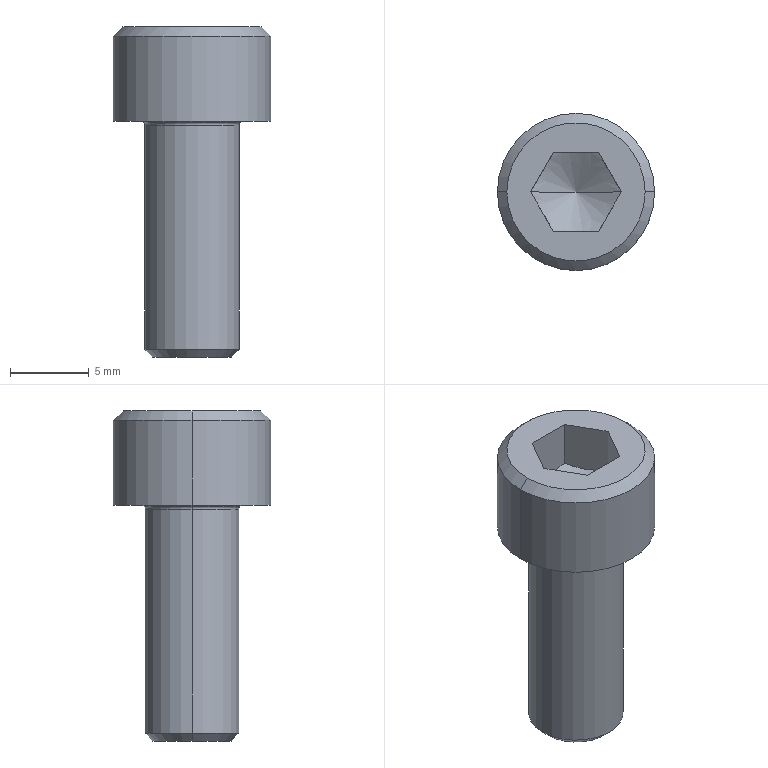Part | Creo | 1 solid | 23 faces | box 10 x 10 x 21 mm | volume 808.86 mm3 | plane 9 | cone 6 | cylinder 4 | torus 4 | commonest cylinder face diameters 6 x2 10 x2
STEP:
#1=CARTESIAN_POINT('',(0.,0.,0.));
#2=DIRECTION('',(0.,0.,1.));
#3=DIRECTION('',(1.,0.,0.));
#4=AXIS2_PLACEMENT_3D('',#1,#2,#3);
#5=CARTESIAN_POINT('',(-133.613,-0.4,-26.828));
#6=VERTEX_POINT('',#5);
#7=CARTESIAN_POINT('',(-135.057,2.1,-26.828));
#8=VERTEX_POINT('',#7);
#9=CARTESIAN_POINT('',(-133.613,-0.4,-26.828));
#10=CARTESIAN_POINT('',(-133.649,-0.3372,-26.848));
#11=CARTESIAN_POINT('',(-133.721,-0.2135,-26.887));
#12=CARTESIAN_POINT('',(-133.824,-0.03475,-26.936));
#13=CARTESIAN_POINT('',(-133.926,0.1409,-26.977));
#14=CARTESIAN_POINT('',(-134.026,0.3156,-27.009));
#15=CARTESIAN_POINT('',(-134.128,0.4922,-27.033));
#16=CARTESIAN_POINT('',(-134.231,0.6704,-27.047));
#17=CARTESIAN_POINT('',(-134.335,0.85,-27.052));
#18=CARTESIAN_POINT('',(-134.439,1.03,-27.047));
#19=CARTESIAN_POINT('',(-134.542,1.208,-27.033));
#20=CARTESIAN_POINT('',(-134.643,1.384,-27.009));
#21=CARTESIAN_POINT('',(-134.744,1.559,-26.977));
#22=CARTESIAN_POINT('',(-134.846,1.735,-26.936));
#23=CARTESIAN_POINT('',(-134.949,1.914,-26.887));
#24=CARTESIAN_POINT('',(-135.02,2.037,-26.848));
#25=CARTESIAN_POINT('',(-135.057,2.1,-26.828));
#26=B_SPLINE_CURVE_WITH_KNOTS('',3,(#9,#10,#11,#12,#13,#14,#15,#16,#17,#18,#19,#20,#21,#22,#23,#24,#25),.UNSPECIFIED.,.F.,.F.,(4,1,1,1,1,1,1,1,1,1,1,1,1,1,4),(0.,0.07143,0.1429,0.2143,0.2857,0.3571,0.4286,0.5,0.5714,0.6429,0.7143,0.7857,0.8571,0.9286,1.),.UNSPECIFIED.);
#27=EDGE_CURVE('',#6,#8,#26,.T.);
#28=ORIENTED_EDGE('',*,*,#27,.F.);
#29=CARTESIAN_POINT('',(-136.5,-0.4,-28.494));
#30=VERTEX_POINT('',#29);
#31=CARTESIAN_POINT('',(-136.5,-0.4,-28.494));
#32=DIRECTION('',(0.866,0.,0.5));
#33=VECTOR('',#32,3.333);
#34=LINE('',#31,#33);
#35=EDGE_CURVE('',#30,#6,#34,.T.);
#36=ORIENTED_EDGE('',*,*,#35,.F.);
#37=CARTESIAN_POINT('',(-139.387,-0.4,-26.828));
#38=VERTEX_POINT('',#37);
#39=CARTESIAN_POINT('',(-136.5,-0.4,-28.494));
#40=DIRECTION('',(-0.866,0.,0.5));
#41=VECTOR('',#40,3.333);
#42=LINE('',#39,#41);
#43=EDGE_CURVE('',#30,#38,#42,.T.);
#44=ORIENTED_EDGE('',*,*,#43,.T.);
#45=CARTESIAN_POINT('',(-137.943,2.1,-26.828));
#46=VERTEX_POINT('',#45);
#47=CARTESIAN_POINT('',(-137.943,2.1,-26.828));
#48=CARTESIAN_POINT('',(-137.98,2.037,-26.848));
#49=CARTESIAN_POINT('',(-138.051,1.914,-26.887));
#50=CARTESIAN_POINT('',(-138.154,1.735,-26.936));
#51=CARTESIAN_POINT('',(-138.256,1.559,-26.977));
#52=CARTESIAN_POINT('',(-138.357,1.384,-27.009));
#53=CARTESIAN_POINT('',(-138.458,1.208,-27.033));
#54=CARTESIAN_POINT('',(-138.561,1.03,-27.047));
#55=CARTESIAN_POINT('',(-138.665,0.85,-27.052));
#56=CARTESIAN_POINT('',(-138.769,0.6704,-27.047));
#57=CARTESIAN_POINT('',(-138.872,0.4922,-27.033));
#58=CARTESIAN_POINT('',(-138.974,0.3156,-27.009));
#59=CARTESIAN_POINT('',(-139.074,0.1409,-26.977));
#60=CARTESIAN_POINT('',(-139.176,-0.03475,-26.936));
#61=CARTESIAN_POINT('',(-139.279,-0.2135,-26.887));
#62=CARTESIAN_POINT('',(-139.351,-0.3372,-26.848));
#63=CARTESIAN_POINT('',(-139.387,-0.4,-26.828));
#64=B_SPLINE_CURVE_WITH_KNOTS('',3,(#47,#48,#49,#50,#51,#52,#53,#54,#55,#56,#57,#58,#59,#60,#61,#62,#63),.UNSPECIFIED.,.F.,.F.,(4,1,1,1,1,1,1,1,1,1,1,1,1,1,4),(0.,0.07143,0.1429,0.2143,0.2857,0.3571,0.4286,0.5,0.5714,0.6429,0.7143,0.7857,0.8571,0.9286,1.),.UNSPECIFIED.);
#65=EDGE_CURVE('',#46,#38,#64,.T.);
#66=ORIENTED_EDGE('',*,*,#65,.F.);
#67=CARTESIAN_POINT('',(-135.057,2.1,-26.828));
#68=CARTESIAN_POINT('',(-135.129,2.1,-26.848));
#69=CARTESIAN_POINT('',(-135.272,2.1,-26.887));
#70=CARTESIAN_POINT('',(-135.478,2.1,-26.936));
#71=CARTESIAN_POINT('',(-135.68,2.1,-26.977));
#72=CARTESIAN_POINT('',(-135.882,2.1,-27.009));
#73=CARTESIAN_POINT('',(-136.086,2.1,-27.033));
#74=CARTESIAN_POINT('',(-136.292,2.1,-27.047));
#75=CARTESIAN_POINT('',(-136.5,2.1,-27.052));
#76=CARTESIAN_POINT('',(-136.708,2.1,-27.047));
#77=CARTESIAN_POINT('',(-136.914,2.1,-27.033));
#78=CARTESIAN_POINT('',(-137.118,2.1,-27.009));
#79=CARTESIAN_POINT('',(-137.32,2.1,-26.977));
#80=CARTESIAN_POINT('',(-137.522,2.1,-26.936));
#81=CARTESIAN_POINT('',(-137.728,2.1,-26.887));
#82=CARTESIAN_POINT('',(-137.871,2.1,-26.848));
#83=CARTESIAN_POINT('',(-137.943,2.1,-26.828));
#84=B_SPLINE_CURVE_WITH_KNOTS('',3,(#67,#68,#69,#70,#71,#72,#73,#74,#75,#76,#77,#78,#79,#80,#81,#82,#83),.UNSPECIFIED.,.F.,.F.,(4,1,1,1,1,1,1,1,1,1,1,1,1,1,4),(0.,0.07143,0.1429,0.2143,0.2857,0.3571,0.4286,0.5,0.5714,0.6429,0.7143,0.7857,0.8571,0.9286,1.),.UNSPECIFIED.);
#85=EDGE_CURVE('',#8,#46,#84,.T.);
#86=ORIENTED_EDGE('',*,*,#85,.F.);
#87=EDGE_LOOP('',(#28,#36,#44,#66,#86));
#88=FACE_OUTER_BOUND('',#87,.F.);
#89=CARTESIAN_POINT('',(-136.5,-0.4,-27.644));
#90=DIRECTION('',(0.,0.,1.));
#91=DIRECTION('',(1.,0.,0.));
#92=AXIS2_PLACEMENT_3D('',#89,#90,#91);
#93=CONICAL_SURFACE('',#92,1.472,60.);
#94=ADVANCED_FACE('',(#88),#93,.F.);
#95=CARTESIAN_POINT('',(-135.057,2.1,-23.828));
#96=VERTEX_POINT('',#95);
#97=CARTESIAN_POINT('',(-133.613,-0.4,-23.828));
#98=VERTEX_POINT('',#97);
#99=CARTESIAN_POINT('',(-135.057,2.1,-23.828));
#100=DIRECTION('',(0.5,-0.866,0.));
#101=VECTOR('',#100,2.887);
#102=LINE('',#99,#101);
#103=EDGE_CURVE('',#96,#98,#102,.T.);
#104=ORIENTED_EDGE('',*,*,#103,.T.);
#105=CARTESIAN_POINT('',(-133.613,-0.4,-23.828));
#106=DIRECTION('',(0.,0.,-1.));
#107=VECTOR('',#106,3.);
#108=LINE('',#105,#107);
#109=EDGE_CURVE('',#98,#6,#108,.T.);
#110=ORIENTED_EDGE('',*,*,#109,.T.);
#111=ORIENTED_EDGE('',*,*,#27,.T.);
#112=CARTESIAN_POINT('',(-135.057,2.1,-23.828));
#113=DIRECTION('',(0.,0.,-1.));
#114=VECTOR('',#113,3.);
#115=LINE('',#112,#114);
#116=EDGE_CURVE('',#96,#8,#115,.T.);
#117=ORIENTED_EDGE('',*,*,#116,.F.);
#118=EDGE_LOOP('',(#104,#110,#111,#117));
#119=FACE_OUTER_BOUND('',#118,.F.);
#120=CARTESIAN_POINT('',(-135.057,2.1,-26.828));
#121=DIRECTION('',(-0.866,-0.5,0.));
#122=DIRECTION('',(0.5,-0.866,0.));
#123=AXIS2_PLACEMENT_3D('',#120,#121,#122);
#124=PLANE('',#123);
#125=ADVANCED_FACE('',(#119),#124,.T.);
#126=CARTESIAN_POINT('',(-132.1,-0.4,-23.828));
#127=VERTEX_POINT('',#126);
#128=CARTESIAN_POINT('',(-140.9,-0.4,-23.828));
#129=VERTEX_POINT('',#128);
#130=CARTESIAN_POINT('',(-136.5,-0.4,-23.828));
#131=DIRECTION('',(0.,0.,1.));
#132=DIRECTION('',(1.,0.,0.));
#133=AXIS2_PLACEMENT_3D('',#130,#131,#132);
#134=CIRCLE('',#133,4.4);
#135=EDGE_CURVE('',#127,#129,#134,.T.);
#136=ORIENTED_EDGE('',*,*,#135,.F.);
#137=CARTESIAN_POINT('',(-136.5,-0.4,-23.828));
#138=DIRECTION('',(0.,0.,1.));
#139=DIRECTION('',(-1.,0.,0.));
#140=AXIS2_PLACEMENT_3D('',#137,#138,#139);
#141=CIRCLE('',#140,4.4);
#142=EDGE_CURVE('',#129,#127,#141,.T.);
#143=ORIENTED_EDGE('',*,*,#142,.F.);
#144=EDGE_LOOP('',(#136,#143));
#145=FACE_OUTER_BOUND('',#144,.F.);
#146=CARTESIAN_POINT('',(-135.057,-2.9,-23.828));
#147=VERTEX_POINT('',#146);
#148=CARTESIAN_POINT('',(-133.613,-0.4,-23.828));
#149=DIRECTION('',(-0.5,-0.866,0.));
#150=VECTOR('',#149,2.887);
#151=LINE('',#148,#150);
#152=EDGE_CURVE('',#98,#147,#151,.T.);
#153=ORIENTED_EDGE('',*,*,#152,.F.);
#154=ORIENTED_EDGE('',*,*,#103,.F.);
#155=CARTESIAN_POINT('',(-137.943,2.1,-23.828));
#156=VERTEX_POINT('',#155);
#157=CARTESIAN_POINT('',(-135.057,2.1,-23.828));
#158=DIRECTION('',(-1.,0.,0.));
#159=VECTOR('',#158,2.887);
#160=LINE('',#157,#159);
#161=EDGE_CURVE('',#96,#156,#160,.T.);
#162=ORIENTED_EDGE('',*,*,#161,.T.);
#163=CARTESIAN_POINT('',(-139.387,-0.4,-23.828));
#164=VERTEX_POINT('',#163);
#165=CARTESIAN_POINT('',(-139.387,-0.4,-23.828));
#166=DIRECTION('',(0.5,0.866,0.));
#167=VECTOR('',#166,2.887);
#168=LINE('',#165,#167);
#169=EDGE_CURVE('',#164,#156,#168,.T.);
#170=ORIENTED_EDGE('',*,*,#169,.F.);
#171=CARTESIAN_POINT('',(-137.943,-2.9,-23.828));
#172=VERTEX_POINT('',#171);
#173=CARTESIAN_POINT('',(-137.943,-2.9,-23.828));
#174=DIRECTION('',(-0.5,0.866,0.));
#175=VECTOR('',#174,2.887);
#176=LINE('',#173,#175);
#177=EDGE_CURVE('',#172,#164,#176,.T.);
#178=ORIENTED_EDGE('',*,*,#177,.F.);
#179=CARTESIAN_POINT('',(-137.943,-2.9,-23.828));
#180=DIRECTION('',(1.,0.,0.));
#181=VECTOR('',#180,2.887);
#182=LINE('',#179,#181);
#183=EDGE_CURVE('',#172,#147,#182,.T.);
#184=ORIENTED_EDGE('',*,*,#183,.T.);
#185=EDGE_LOOP('',(#153,#154,#162,#170,#178,#184));
#186=FACE_BOUND('',#185,.F.);
#187=CARTESIAN_POINT('',(-136.5,-0.4,-23.828));
#188=DIRECTION('',(0.,0.,1.));
#189=DIRECTION('',(1.,0.,0.));
#190=AXIS2_PLACEMENT_3D('',#187,#188,#189);
#191=PLANE('',#190);
#192=ADVANCED_FACE('',(#145,#186),#191,.T.);
#193=CARTESIAN_POINT('',(-131.5,-0.4,-24.427));
#194=VERTEX_POINT('',#193);
#195=CARTESIAN_POINT('',(-141.5,-0.4,-24.427));
#196=VERTEX_POINT('',#195);
#197=CARTESIAN_POINT('',(-136.5,-0.4,-24.427));
#198=DIRECTION('',(0.,0.,1.));
#199=DIRECTION('',(1.,0.,0.));
#200=AXIS2_PLACEMENT_3D('',#197,#198,#199);
#201=CIRCLE('',#200,5.);
#202=EDGE_CURVE('',#194,#196,#201,.T.);
#203=ORIENTED_EDGE('',*,*,#202,.F.);
#204=CARTESIAN_POINT('',(-132.1,-0.4,-23.828));
#205=DIRECTION('',(0.7071,0.,-0.7071));
#206=VECTOR('',#205,0.8485);
#207=LINE('',#204,#206);
#208=EDGE_CURVE('',#127,#194,#207,.T.);
#209=ORIENTED_EDGE('',*,*,#208,.F.);
#210=ORIENTED_EDGE('',*,*,#135,.T.);
#211=CARTESIAN_POINT('',(-140.9,-0.4,-23.828));
#212=DIRECTION('',(-0.7071,0.,-0.7071));
#213=VECTOR('',#212,0.8485);
#214=LINE('',#211,#213);
#215=EDGE_CURVE('',#129,#196,#214,.T.);
#216=ORIENTED_EDGE('',*,*,#215,.T.);
#217=EDGE_LOOP('',(#203,#209,#210,#216));
#218=FACE_OUTER_BOUND('',#217,.F.);
#219=CARTESIAN_POINT('',(-136.5,-0.4,-24.128));
#220=DIRECTION('',(0.,0.,-1.));
#221=DIRECTION('',(-1.,0.,0.));
#222=AXIS2_PLACEMENT_3D('',#219,#220,#221);
#223=CONICAL_SURFACE('',#222,4.7,45.);
#224=ADVANCED_FACE('',(#218),#223,.T.);
#225=ORIENTED_EDGE('',*,*,#202,.T.);
#226=CARTESIAN_POINT('',(-141.5,-0.4,-29.828));
#227=VERTEX_POINT('',#226);
#228=CARTESIAN_POINT('',(-141.5,-0.4,-29.828));
#229=DIRECTION('',(0.,0.,1.));
#230=VECTOR('',#229,5.4);
#231=LINE('',#228,#230);
#232=EDGE_CURVE('',#227,#196,#231,.T.);
#233=ORIENTED_EDGE('',*,*,#232,.F.);
#234=CARTESIAN_POINT('',(-131.5,-0.4,-29.828));
#235=VERTEX_POINT('',#234);
#236=CARTESIAN_POINT('',(-136.5,-0.4,-29.828));
#237=DIRECTION('',(0.,0.,-1.));
#238=DIRECTION('',(-1.,0.,0.));
#239=AXIS2_PLACEMENT_3D('',#236,#237,#238);
#240=CIRCLE('',#239,5.);
#241=EDGE_CURVE('',#227,#235,#240,.T.);
#242=ORIENTED_EDGE('',*,*,#241,.T.);
#243=CARTESIAN_POINT('',(-131.5,-0.4,-29.828));
#244=DIRECTION('',(0.,0.,1.));
#245=VECTOR('',#244,5.4);
#246=LINE('',#243,#245);
#247=EDGE_CURVE('',#235,#194,#246,.T.);
#248=ORIENTED_EDGE('',*,*,#247,.T.);
#249=EDGE_LOOP('',(#225,#233,#242,#248));
#250=FACE_OUTER_BOUND('',#249,.F.);
#251=CARTESIAN_POINT('',(-136.5,-0.4,-29.828));
#252=DIRECTION('',(0.,0.,1.));
#253=DIRECTION('',(1.,0.,0.));
#254=AXIS2_PLACEMENT_3D('',#251,#252,#253);
#255=CYLINDRICAL_SURFACE('',#254,5.);
#256=ADVANCED_FACE('',(#250),#255,.T.);
#257=CARTESIAN_POINT('',(-136.5,-0.4,-24.427));
#258=DIRECTION('',(0.,0.,1.));
#259=DIRECTION('',(-1.,0.,0.));
#260=AXIS2_PLACEMENT_3D('',#257,#258,#259);
#261=CIRCLE('',#260,5.);
#262=EDGE_CURVE('',#196,#194,#261,.T.);
#263=ORIENTED_EDGE('',*,*,#262,.T.);
#264=ORIENTED_EDGE('',*,*,#247,.F.);
#265=CARTESIAN_POINT('',(-136.5,-0.4,-29.828));
#266=DIRECTION('',(0.,0.,-1.));
#267=DIRECTION('',(1.,0.,0.));
#268=AXIS2_PLACEMENT_3D('',#265,#266,#267);
#269=CIRCLE('',#268,5.);
#270=EDGE_CURVE('',#235,#227,#269,.T.);
#271=ORIENTED_EDGE('',*,*,#270,.T.);
#272=ORIENTED_EDGE('',*,*,#232,.T.);
#273=EDGE_LOOP('',(#263,#264,#271,#272));
#274=FACE_OUTER_BOUND('',#273,.F.);
#275=CARTESIAN_POINT('',(-136.5,-0.4,-29.828));
#276=DIRECTION('',(0.,0.,1.));
#277=DIRECTION('',(1.,0.,0.));
#278=AXIS2_PLACEMENT_3D('',#275,#276,#277);
#279=CYLINDRICAL_SURFACE('',#278,5.);
#280=ADVANCED_FACE('',(#274),#279,.T.);
#281=ORIENTED_EDGE('',*,*,#262,.F.);
#282=ORIENTED_EDGE('',*,*,#215,.F.);
#283=ORIENTED_EDGE('',*,*,#142,.T.);
#284=ORIENTED_EDGE('',*,*,#208,.T.);
#285=EDGE_LOOP('',(#281,#282,#283,#284));
#286=FACE_OUTER_BOUND('',#285,.F.);
#287=CARTESIAN_POINT('',(-136.5,-0.4,-24.128));
#288=DIRECTION('',(0.,0.,-1.));
#289=DIRECTION('',(-1.,0.,0.));
#290=AXIS2_PLACEMENT_3D('',#287,#288,#289);
#291=CONICAL_SURFACE('',#290,4.7,45.);
#292=ADVANCED_FACE('',(#286),#291,.T.);
#293=ORIENTED_EDGE('',*,*,#270,.F.);
#294=ORIENTED_EDGE('',*,*,#241,.F.);
#295=EDGE_LOOP('',(#293,#294));
#296=FACE_OUTER_BOUND('',#295,.F.);
#297=CARTESIAN_POINT('',(-133.25,-0.4,-29.828));
#298=VERTEX_POINT('',#297);
#299=CARTESIAN_POINT('',(-139.75,-0.4,-29.828));
#300=VERTEX_POINT('',#299);
#301=CARTESIAN_POINT('',(-136.5,-0.4,-29.828));
#302=DIRECTION('',(0.,0.,1.));
#303=DIRECTION('',(1.,0.,0.));
#304=AXIS2_PLACEMENT_3D('',#301,#302,#303);
#305=CIRCLE('',#304,3.25);
#306=EDGE_CURVE('',#298,#300,#305,.T.);
#307=ORIENTED_EDGE('',*,*,#306,.F.);
#308=CARTESIAN_POINT('',(-136.5,-0.4,-29.828));
#309=DIRECTION('',(0.,0.,1.));
#310=DIRECTION('',(-1.,0.,0.));
#311=AXIS2_PLACEMENT_3D('',#308,#309,#310);
#312=CIRCLE('',#311,3.25);
#313=EDGE_CURVE('',#300,#298,#312,.T.);
#314=ORIENTED_EDGE('',*,*,#313,.F.);
#315=EDGE_LOOP('',(#307,#314));
#316=FACE_BOUND('',#315,.F.);
#317=CARTESIAN_POINT('',(-136.5,-0.4,-29.828));
#318=DIRECTION('',(0.,0.,1.));
#319=DIRECTION('',(1.,0.,0.));
#320=AXIS2_PLACEMENT_3D('',#317,#318,#319);
#321=PLANE('',#320);
#322=ADVANCED_FACE('',(#296,#316),#321,.F.);
#323=ORIENTED_EDGE('',*,*,#306,.T.);
#324=CARTESIAN_POINT('',(-139.573,-0.4,-29.901));
#325=VERTEX_POINT('',#324);
#326=CARTESIAN_POINT('',(-139.75,-0.4,-30.078));
#327=DIRECTION('',(0.,1.,0.));
#328=DIRECTION('',(0.,0.,1.));
#329=AXIS2_PLACEMENT_3D('',#326,#327,#328);
#330=CIRCLE('',#329,0.25);
#331=EDGE_CURVE('',#300,#325,#330,.T.);
#332=ORIENTED_EDGE('',*,*,#331,.T.);
#333=CARTESIAN_POINT('',(-133.427,-0.4,-29.901));
#334=VERTEX_POINT('',#333);
#335=CARTESIAN_POINT('',(-136.5,-0.4,-29.901));
#336=DIRECTION('',(0.,0.,1.));
#337=DIRECTION('',(1.,0.,0.));
#338=AXIS2_PLACEMENT_3D('',#335,#336,#337);
#339=CIRCLE('',#338,3.073);
#340=EDGE_CURVE('',#334,#325,#339,.T.);
#341=ORIENTED_EDGE('',*,*,#340,.F.);
#342=CARTESIAN_POINT('',(-133.25,-0.4,-30.078));
#343=DIRECTION('',(0.,-1.,0.));
#344=DIRECTION('',(0.,0.,1.));
#345=AXIS2_PLACEMENT_3D('',#342,#343,#344);
#346=CIRCLE('',#345,0.25);
#347=EDGE_CURVE('',#298,#334,#346,.T.);
#348=ORIENTED_EDGE('',*,*,#347,.F.);
#349=EDGE_LOOP('',(#323,#332,#341,#348));
#350=FACE_OUTER_BOUND('',#349,.F.);
#351=CARTESIAN_POINT('',(-136.5,-0.4,-30.078));
#352=DIRECTION('',(0.,0.,1.));
#353=DIRECTION('',(1.,0.,0.));
#354=AXIS2_PLACEMENT_3D('',#351,#352,#353);
#355=TOROIDAL_SURFACE('',#354,3.25,0.25);
#356=ADVANCED_FACE('',(#350),#355,.F.);
#357=ORIENTED_EDGE('',*,*,#313,.T.);
#358=ORIENTED_EDGE('',*,*,#347,.T.);
#359=CARTESIAN_POINT('',(-136.5,-0.4,-29.901));
#360=DIRECTION('',(0.,0.,1.));
#361=DIRECTION('',(-1.,0.,0.));
#362=AXIS2_PLACEMENT_3D('',#359,#360,#361);
#363=CIRCLE('',#362,3.073);
#364=EDGE_CURVE('',#325,#334,#363,.T.);
#365=ORIENTED_EDGE('',*,*,#364,.F.);
#366=ORIENTED_EDGE('',*,*,#331,.F.);
#367=EDGE_LOOP('',(#357,#358,#365,#366));
#368=FACE_OUTER_BOUND('',#367,.F.);
#369=CARTESIAN_POINT('',(-136.5,-0.4,-30.078));
#370=DIRECTION('',(0.,0.,1.));
#371=DIRECTION('',(1.,0.,0.));
#372=AXIS2_PLACEMENT_3D('',#369,#370,#371);
#373=TOROIDAL_SURFACE('',#372,3.25,0.25);
#374=ADVANCED_FACE('',(#368),#373,.F.);
#375=CARTESIAN_POINT('',(-139.5,-0.4,-30.078));
#376=VERTEX_POINT('',#375);
#377=CARTESIAN_POINT('',(-133.5,-0.4,-30.078));
#378=VERTEX_POINT('',#377);
#379=CARTESIAN_POINT('',(-136.5,-0.4,-30.078));
#380=DIRECTION('',(0.,0.,1.));
#381=DIRECTION('',(-1.,0.,0.));
#382=AXIS2_PLACEMENT_3D('',#379,#380,#381);
#383=CIRCLE('',#382,3.);
#384=EDGE_CURVE('',#376,#378,#383,.T.);
#385=ORIENTED_EDGE('',*,*,#384,.F.);
#386=CARTESIAN_POINT('',(-139.75,-0.4,-30.078));
#387=DIRECTION('',(0.,1.,0.));
#388=DIRECTION('',(0.7071,0.,0.7071));
#389=AXIS2_PLACEMENT_3D('',#386,#387,#388);
#390=CIRCLE('',#389,0.25);
#391=EDGE_CURVE('',#325,#376,#390,.T.);
#392=ORIENTED_EDGE('',*,*,#391,.F.);
#393=ORIENTED_EDGE('',*,*,#364,.T.);
#394=CARTESIAN_POINT('',(-133.25,-0.4,-30.078));
#395=DIRECTION('',(0.,-1.,0.));
#396=DIRECTION('',(-0.7071,0.,0.7071));
#397=AXIS2_PLACEMENT_3D('',#394,#395,#396);
#398=CIRCLE('',#397,0.25);
#399=EDGE_CURVE('',#334,#378,#398,.T.);
#400=ORIENTED_EDGE('',*,*,#399,.T.);
#401=EDGE_LOOP('',(#385,#392,#393,#400));
#402=FACE_OUTER_BOUND('',#401,.F.);
#403=CARTESIAN_POINT('',(-136.5,-0.4,-30.078));
#404=DIRECTION('',(0.,0.,1.));
#405=DIRECTION('',(1.,0.,0.));
#406=AXIS2_PLACEMENT_3D('',#403,#404,#405);
#407=TOROIDAL_SURFACE('',#406,3.25,0.25);
#408=ADVANCED_FACE('',(#402),#407,.F.);
#409=CARTESIAN_POINT('',(-133.5,-0.4,-44.328));
#410=VERTEX_POINT('',#409);
#411=CARTESIAN_POINT('',(-139.5,-0.4,-44.328));
#412=VERTEX_POINT('',#411);
#413=CARTESIAN_POINT('',(-136.5,-0.4,-44.328));
#414=DIRECTION('',(0.,0.,-1.));
#415=DIRECTION('',(1.,0.,0.));
#416=AXIS2_PLACEMENT_3D('',#413,#414,#415);
#417=CIRCLE('',#416,3.);
#418=EDGE_CURVE('',#410,#412,#417,.T.);
#419=ORIENTED_EDGE('',*,*,#418,.T.);
#420=CARTESIAN_POINT('',(-139.5,-0.4,-44.328));
#421=DIRECTION('',(0.,0.,1.));
#422=VECTOR('',#421,14.25);
#423=LINE('',#420,#422);
#424=EDGE_CURVE('',#412,#376,#423,.T.);
#425=ORIENTED_EDGE('',*,*,#424,.T.);
#426=ORIENTED_EDGE('',*,*,#384,.T.);
#427=CARTESIAN_POINT('',(-133.5,-0.4,-44.328));
#428=DIRECTION('',(0.,0.,1.));
#429=VECTOR('',#428,14.25);
#430=LINE('',#427,#429);
#431=EDGE_CURVE('',#410,#378,#430,.T.);
#432=ORIENTED_EDGE('',*,*,#431,.F.);
#433=EDGE_LOOP('',(#419,#425,#426,#432));
#434=FACE_OUTER_BOUND('',#433,.F.);
#435=CARTESIAN_POINT('',(-136.5,-0.4,-44.828));
#436=DIRECTION('',(0.,0.,1.));
#437=DIRECTION('',(1.,0.,0.));
#438=AXIS2_PLACEMENT_3D('',#435,#436,#437);
#439=CYLINDRICAL_SURFACE('',#438,3.);
#440=ADVANCED_FACE('',(#434),#439,.T.);
#441=CARTESIAN_POINT('',(-134.,-0.4,-44.828));
#442=VERTEX_POINT('',#441);
#443=CARTESIAN_POINT('',(-139.,-0.4,-44.828));
#444=VERTEX_POINT('',#443);
#445=CARTESIAN_POINT('',(-136.5,-0.4,-44.828));
#446=DIRECTION('',(0.,0.,-1.));
#447=DIRECTION('',(1.,0.,0.));
#448=AXIS2_PLACEMENT_3D('',#445,#446,#447);
#449=CIRCLE('',#448,2.5);
#450=EDGE_CURVE('',#442,#444,#449,.T.);
#451=ORIENTED_EDGE('',*,*,#450,.T.);
#452=CARTESIAN_POINT('',(-139.,-0.4,-44.828));
#453=DIRECTION('',(-0.7071,0.,0.7071));
#454=VECTOR('',#453,0.7071);
#455=LINE('',#452,#454);
#456=EDGE_CURVE('',#444,#412,#455,.T.);
#457=ORIENTED_EDGE('',*,*,#456,.T.);
#458=ORIENTED_EDGE('',*,*,#418,.F.);
#459=CARTESIAN_POINT('',(-134.,-0.4,-44.828));
#460=DIRECTION('',(0.7071,0.,0.7071));
#461=VECTOR('',#460,0.7071);
#462=LINE('',#459,#461);
#463=EDGE_CURVE('',#442,#410,#462,.T.);
#464=ORIENTED_EDGE('',*,*,#463,.F.);
#465=EDGE_LOOP('',(#451,#457,#458,#464));
#466=FACE_OUTER_BOUND('',#465,.F.);
#467=CARTESIAN_POINT('',(-136.5,-0.4,-44.578));
#468=DIRECTION('',(0.,0.,1.));
#469=DIRECTION('',(1.,0.,0.));
#470=AXIS2_PLACEMENT_3D('',#467,#468,#469);
#471=CONICAL_SURFACE('',#470,2.75,45.);
#472=ADVANCED_FACE('',(#466),#471,.T.);
#473=ORIENTED_EDGE('',*,*,#450,.F.);
#474=CARTESIAN_POINT('',(-136.5,-0.4,-44.828));
#475=DIRECTION('',(0.,0.,-1.));
#476=DIRECTION('',(-1.,0.,0.));
#477=AXIS2_PLACEMENT_3D('',#474,#475,#476);
#478=CIRCLE('',#477,2.5);
#479=EDGE_CURVE('',#444,#442,#478,.T.);
#480=ORIENTED_EDGE('',*,*,#479,.F.);
#481=EDGE_LOOP('',(#473,#480));
#482=FACE_OUTER_BOUND('',#481,.F.);
#483=CARTESIAN_POINT('',(-136.5,-0.4,-44.828));
#484=DIRECTION('',(0.,0.,1.));
#485=DIRECTION('',(1.,0.,0.));
#486=AXIS2_PLACEMENT_3D('',#483,#484,#485);
#487=PLANE('',#486);
#488=ADVANCED_FACE('',(#482),#487,.F.);
#489=ORIENTED_EDGE('',*,*,#479,.T.);
#490=ORIENTED_EDGE('',*,*,#463,.T.);
#491=CARTESIAN_POINT('',(-136.5,-0.4,-44.328));
#492=DIRECTION('',(0.,0.,-1.));
#493=DIRECTION('',(-1.,0.,0.));
#494=AXIS2_PLACEMENT_3D('',#491,#492,#493);
#495=CIRCLE('',#494,3.);
#496=EDGE_CURVE('',#412,#410,#495,.T.);
#497=ORIENTED_EDGE('',*,*,#496,.F.);
#498=ORIENTED_EDGE('',*,*,#456,.F.);
#499=EDGE_LOOP('',(#489,#490,#497,#498));
#500=FACE_OUTER_BOUND('',#499,.F.);
#501=CARTESIAN_POINT('',(-136.5,-0.4,-44.578));
#502=DIRECTION('',(0.,0.,1.));
#503=DIRECTION('',(1.,0.,0.));
#504=AXIS2_PLACEMENT_3D('',#501,#502,#503);
#505=CONICAL_SURFACE('',#504,2.75,45.);
#506=ADVANCED_FACE('',(#500),#505,.T.);
#507=ORIENTED_EDGE('',*,*,#496,.T.);
#508=ORIENTED_EDGE('',*,*,#431,.T.);
#509=CARTESIAN_POINT('',(-136.5,-0.4,-30.078));
#510=DIRECTION('',(0.,0.,1.));
#511=DIRECTION('',(1.,0.,0.));
#512=AXIS2_PLACEMENT_3D('',#509,#510,#511);
#513=CIRCLE('',#512,3.);
#514=EDGE_CURVE('',#378,#376,#513,.T.);
#515=ORIENTED_EDGE('',*,*,#514,.T.);
#516=ORIENTED_EDGE('',*,*,#424,.F.);
#517=EDGE_LOOP('',(#507,#508,#515,#516));
#518=FACE_OUTER_BOUND('',#517,.F.);
#519=CARTESIAN_POINT('',(-136.5,-0.4,-44.828));
#520=DIRECTION('',(0.,0.,1.));
#521=DIRECTION('',(1.,0.,0.));
#522=AXIS2_PLACEMENT_3D('',#519,#520,#521);
#523=CYLINDRICAL_SURFACE('',#522,3.);
#524=ADVANCED_FACE('',(#518),#523,.T.);
#525=ORIENTED_EDGE('',*,*,#514,.F.);
#526=ORIENTED_EDGE('',*,*,#399,.F.);
#527=ORIENTED_EDGE('',*,*,#340,.T.);
#528=ORIENTED_EDGE('',*,*,#391,.T.);
#529=EDGE_LOOP('',(#525,#526,#527,#528));
#530=FACE_OUTER_BOUND('',#529,.F.);
#531=CARTESIAN_POINT('',(-136.5,-0.4,-30.078));
#532=DIRECTION('',(0.,0.,1.));
#533=DIRECTION('',(1.,0.,0.));
#534=AXIS2_PLACEMENT_3D('',#531,#532,#533);
#535=TOROIDAL_SURFACE('',#534,3.25,0.25);
#536=ADVANCED_FACE('',(#530),#535,.F.);
#537=ORIENTED_EDGE('',*,*,#152,.T.);
#538=CARTESIAN_POINT('',(-135.057,-2.9,-26.828));
#539=VERTEX_POINT('',#538);
#540=CARTESIAN_POINT('',(-135.057,-2.9,-23.828));
#541=DIRECTION('',(0.,0.,-1.));
#542=VECTOR('',#541,3.);
#543=LINE('',#540,#542);
#544=EDGE_CURVE('',#147,#539,#543,.T.);
#545=ORIENTED_EDGE('',*,*,#544,.T.);
#546=CARTESIAN_POINT('',(-135.057,-2.9,-26.828));
#547=CARTESIAN_POINT('',(-135.02,-2.837,-26.848));
#548=CARTESIAN_POINT('',(-134.949,-2.714,-26.887));
#549=CARTESIAN_POINT('',(-134.846,-2.535,-26.936));
#550=CARTESIAN_POINT('',(-134.744,-2.359,-26.977));
#551=CARTESIAN_POINT('',(-134.643,-2.184,-27.009));
#552=CARTESIAN_POINT('',(-134.542,-2.008,-27.033));
#553=CARTESIAN_POINT('',(-134.439,-1.83,-27.047));
#554=CARTESIAN_POINT('',(-134.335,-1.65,-27.052));
#555=CARTESIAN_POINT('',(-134.231,-1.47,-27.047));
#556=CARTESIAN_POINT('',(-134.128,-1.292,-27.033));
#557=CARTESIAN_POINT('',(-134.026,-1.116,-27.009));
#558=CARTESIAN_POINT('',(-133.926,-0.9409,-26.977));
#559=CARTESIAN_POINT('',(-133.824,-0.7652,-26.936));
#560=CARTESIAN_POINT('',(-133.721,-0.5865,-26.887));
#561=CARTESIAN_POINT('',(-133.649,-0.4628,-26.848));
#562=CARTESIAN_POINT('',(-133.613,-0.4,-26.828));
#563=B_SPLINE_CURVE_WITH_KNOTS('',3,(#546,#547,#548,#549,#550,#551,#552,#553,#554,#555,#556,#557,#558,#559,#560,#561,#562),.UNSPECIFIED.,.F.,.F.,(4,1,1,1,1,1,1,1,1,1,1,1,1,1,4),(0.,0.07143,0.1429,0.2143,0.2857,0.3571,0.4286,0.5,0.5714,0.6429,0.7143,0.7857,0.8571,0.9286,1.),.UNSPECIFIED.);
#564=EDGE_CURVE('',#539,#6,#563,.T.);
#565=ORIENTED_EDGE('',*,*,#564,.T.);
#566=ORIENTED_EDGE('',*,*,#109,.F.);
#567=EDGE_LOOP('',(#537,#545,#565,#566));
#568=FACE_OUTER_BOUND('',#567,.F.);
#569=CARTESIAN_POINT('',(-133.613,-0.4,-26.828));
#570=DIRECTION('',(-0.866,0.5,0.));
#571=DIRECTION('',(-0.5,-0.866,0.));
#572=AXIS2_PLACEMENT_3D('',#569,#570,#571);
#573=PLANE('',#572);
#574=ADVANCED_FACE('',(#568),#573,.T.);
#575=ORIENTED_EDGE('',*,*,#183,.F.);
#576=CARTESIAN_POINT('',(-137.943,-2.9,-26.828));
#577=VERTEX_POINT('',#576);
#578=CARTESIAN_POINT('',(-137.943,-2.9,-23.828));
#579=DIRECTION('',(0.,0.,-1.));
#580=VECTOR('',#579,3.);
#581=LINE('',#578,#580);
#582=EDGE_CURVE('',#172,#577,#581,.T.);
#583=ORIENTED_EDGE('',*,*,#582,.T.);
#584=CARTESIAN_POINT('',(-137.943,-2.9,-26.828));
#585=CARTESIAN_POINT('',(-137.871,-2.9,-26.848));
#586=CARTESIAN_POINT('',(-137.728,-2.9,-26.887));
#587=CARTESIAN_POINT('',(-137.522,-2.9,-26.936));
#588=CARTESIAN_POINT('',(-137.32,-2.9,-26.977));
#589=CARTESIAN_POINT('',(-137.118,-2.9,-27.009));
#590=CARTESIAN_POINT('',(-136.914,-2.9,-27.033));
#591=CARTESIAN_POINT('',(-136.708,-2.9,-27.047));
#592=CARTESIAN_POINT('',(-136.5,-2.9,-27.052));
#593=CARTESIAN_POINT('',(-136.292,-2.9,-27.047));
#594=CARTESIAN_POINT('',(-136.086,-2.9,-27.033));
#595=CARTESIAN_POINT('',(-135.882,-2.9,-27.009));
#596=CARTESIAN_POINT('',(-135.68,-2.9,-26.977));
#597=CARTESIAN_POINT('',(-135.478,-2.9,-26.936));
#598=CARTESIAN_POINT('',(-135.272,-2.9,-26.887));
#599=CARTESIAN_POINT('',(-135.129,-2.9,-26.848));
#600=CARTESIAN_POINT('',(-135.057,-2.9,-26.828));
#601=B_SPLINE_CURVE_WITH_KNOTS('',3,(#584,#585,#586,#587,#588,#589,#590,#591,#592,#593,#594,#595,#596,#597,#598,#599,#600),.UNSPECIFIED.,.F.,.F.,(4,1,1,1,1,1,1,1,1,1,1,1,1,1,4),(0.,0.07143,0.1429,0.2143,0.2857,0.3571,0.4286,0.5,0.5714,0.6429,0.7143,0.7857,0.8571,0.9286,1.),.UNSPECIFIED.);
#602=EDGE_CURVE('',#577,#539,#601,.T.);
#603=ORIENTED_EDGE('',*,*,#602,.T.);
#604=ORIENTED_EDGE('',*,*,#544,.F.);
#605=EDGE_LOOP('',(#575,#583,#603,#604));
#606=FACE_OUTER_BOUND('',#605,.F.);
#607=CARTESIAN_POINT('',(-135.057,-2.9,-26.828));
#608=DIRECTION('',(0.,1.,0.));
#609=DIRECTION('',(0.,0.,1.));
#610=AXIS2_PLACEMENT_3D('',#607,#608,#609);
#611=PLANE('',#610);
#612=ADVANCED_FACE('',(#606),#611,.T.);
#613=ORIENTED_EDGE('',*,*,#177,.T.);
#614=CARTESIAN_POINT('',(-139.387,-0.4,-23.828));
#615=DIRECTION('',(0.,0.,-1.));
#616=VECTOR('',#615,3.);
#617=LINE('',#614,#616);
#618=EDGE_CURVE('',#164,#38,#617,.T.);
#619=ORIENTED_EDGE('',*,*,#618,.T.);
#620=CARTESIAN_POINT('',(-139.387,-0.4,-26.828));
#621=CARTESIAN_POINT('',(-139.351,-0.4628,-26.848));
#622=CARTESIAN_POINT('',(-139.279,-0.5865,-26.887));
#623=CARTESIAN_POINT('',(-139.176,-0.7652,-26.936));
#624=CARTESIAN_POINT('',(-139.074,-0.9409,-26.977));
#625=CARTESIAN_POINT('',(-138.974,-1.116,-27.009));
#626=CARTESIAN_POINT('',(-138.872,-1.292,-27.033));
#627=CARTESIAN_POINT('',(-138.769,-1.47,-27.047));
#628=CARTESIAN_POINT('',(-138.665,-1.65,-27.052));
#629=CARTESIAN_POINT('',(-138.561,-1.83,-27.047));
#630=CARTESIAN_POINT('',(-138.458,-2.008,-27.033));
#631=CARTESIAN_POINT('',(-138.357,-2.184,-27.009));
#632=CARTESIAN_POINT('',(-138.256,-2.359,-26.977));
#633=CARTESIAN_POINT('',(-138.154,-2.535,-26.936));
#634=CARTESIAN_POINT('',(-138.051,-2.714,-26.887));
#635=CARTESIAN_POINT('',(-137.98,-2.837,-26.848));
#636=CARTESIAN_POINT('',(-137.943,-2.9,-26.828));
#637=B_SPLINE_CURVE_WITH_KNOTS('',3,(#620,#621,#622,#623,#624,#625,#626,#627,#628,#629,#630,#631,#632,#633,#634,#635,#636),.UNSPECIFIED.,.F.,.F.,(4,1,1,1,1,1,1,1,1,1,1,1,1,1,4),(0.,0.07143,0.1429,0.2143,0.2857,0.3571,0.4286,0.5,0.5714,0.6429,0.7143,0.7857,0.8571,0.9286,1.),.UNSPECIFIED.);
#638=EDGE_CURVE('',#38,#577,#637,.T.);
#639=ORIENTED_EDGE('',*,*,#638,.T.);
#640=ORIENTED_EDGE('',*,*,#582,.F.);
#641=EDGE_LOOP('',(#613,#619,#639,#640));
#642=FACE_OUTER_BOUND('',#641,.F.);
#643=CARTESIAN_POINT('',(-137.943,-2.9,-26.828));
#644=DIRECTION('',(0.866,0.5,0.));
#645=DIRECTION('',(-0.5,0.866,0.));
#646=AXIS2_PLACEMENT_3D('',#643,#644,#645);
#647=PLANE('',#646);
#648=ADVANCED_FACE('',(#642),#647,.T.);
#649=ORIENTED_EDGE('',*,*,#169,.T.);
#650=CARTESIAN_POINT('',(-137.943,2.1,-23.828));
#651=DIRECTION('',(0.,0.,-1.));
#652=VECTOR('',#651,3.);
#653=LINE('',#650,#652);
#654=EDGE_CURVE('',#156,#46,#653,.T.);
#655=ORIENTED_EDGE('',*,*,#654,.T.);
#656=ORIENTED_EDGE('',*,*,#65,.T.);
#657=ORIENTED_EDGE('',*,*,#618,.F.);
#658=EDGE_LOOP('',(#649,#655,#656,#657));
#659=FACE_OUTER_BOUND('',#658,.F.);
#660=CARTESIAN_POINT('',(-139.387,-0.4,-26.828));
#661=DIRECTION('',(0.866,-0.5,0.));
#662=DIRECTION('',(0.5,0.866,0.));
#663=AXIS2_PLACEMENT_3D('',#660,#661,#662);
#664=PLANE('',#663);
#665=ADVANCED_FACE('',(#659),#664,.T.);
#666=ORIENTED_EDGE('',*,*,#161,.F.);
#667=ORIENTED_EDGE('',*,*,#116,.T.);
#668=ORIENTED_EDGE('',*,*,#85,.T.);
#669=ORIENTED_EDGE('',*,*,#654,.F.);
#670=EDGE_LOOP('',(#666,#667,#668,#669));
#671=FACE_OUTER_BOUND('',#670,.F.);
#672=CARTESIAN_POINT('',(-137.943,2.1,-26.828));
#673=DIRECTION('',(0.,-1.,0.));
#674=DIRECTION('',(0.,0.,-1.));
#675=AXIS2_PLACEMENT_3D('',#672,#673,#674);
#676=PLANE('',#675);
#677=ADVANCED_FACE('',(#671),#676,.T.);
#678=ORIENTED_EDGE('',*,*,#638,.F.);
#679=ORIENTED_EDGE('',*,*,#43,.F.);
#680=ORIENTED_EDGE('',*,*,#35,.T.);
#681=ORIENTED_EDGE('',*,*,#564,.F.);
#682=ORIENTED_EDGE('',*,*,#602,.F.);
#683=EDGE_LOOP('',(#678,#679,#680,#681,#682));
#684=FACE_OUTER_BOUND('',#683,.F.);
#685=CARTESIAN_POINT('',(-136.5,-0.4,-27.644));
#686=DIRECTION('',(0.,0.,1.));
#687=DIRECTION('',(1.,0.,0.));
#688=AXIS2_PLACEMENT_3D('',#685,#686,#687);
#689=CONICAL_SURFACE('',#688,1.472,60.);
#690=ADVANCED_FACE('',(#684),#689,.F.);
#691=CLOSED_SHELL('',(#94,#125,#192,#224,#256,#280,#292,#322,#356,#374,#408,#440,#472,#488,#506,#524,#536,#574,#612,#648,#665,#677,#690));
#692=MANIFOLD_SOLID_BREP('',#691);
#693=(LENGTH_UNIT()NAMED_UNIT(*)SI_UNIT(.MILLI.,.METRE.));
#694=UNCERTAINTY_MEASURE_WITH_UNIT(LENGTH_MEASURE(0.002532),#693,'','');
#695=(NAMED_UNIT(*)PLANE_ANGLE_UNIT()SI_UNIT($,.RADIAN.));
#696=PLANE_ANGLE_MEASURE_WITH_UNIT(PLANE_ANGLE_MEASURE(0.01745),#695);
#697=(CONVERSION_BASED_UNIT('DEGREE',#696)NAMED_UNIT(*)PLANE_ANGLE_UNIT());
#698=(NAMED_UNIT(*)SI_UNIT($,.STERADIAN.)SOLID_ANGLE_UNIT());
#699=(GEOMETRIC_REPRESENTATION_CONTEXT(3)GLOBAL_UNCERTAINTY_ASSIGNED_CONTEXT((#694))GLOBAL_UNIT_ASSIGNED_CONTEXT((#693,#697,#698))REPRESENTATION_CONTEXT('',''));
#700=ADVANCED_BREP_SHAPE_REPRESENTATION('',(#4,#692),#699);